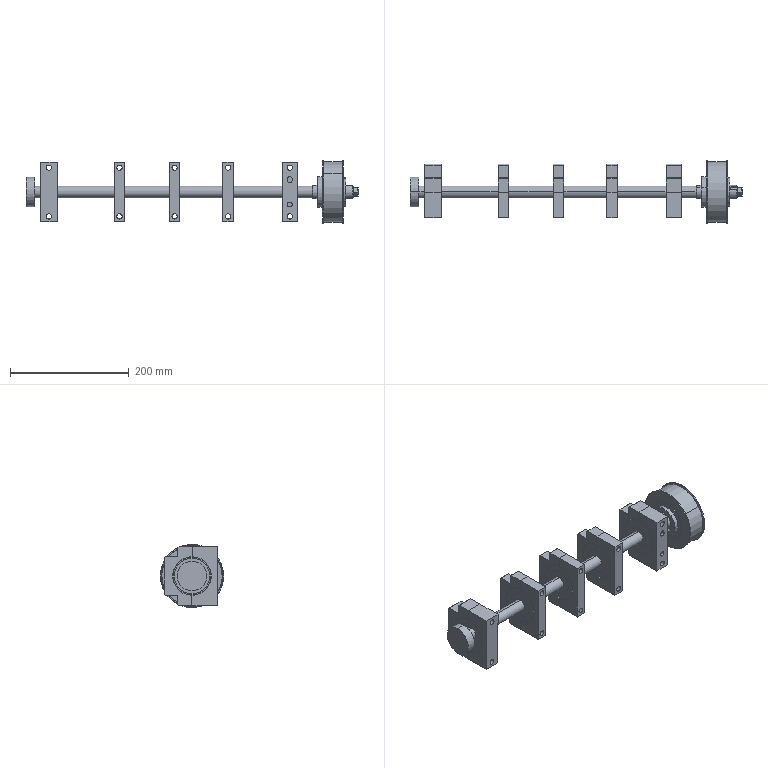Part | SolidWorks | 20 solids | 562 faces | box 559.6 x 107 x 107 mm | volume 1279109 mm3 | cylinder 264 | plane 232 | cone 46 | torus 10 | spline 10 | commonest cylinder face diameters 4 x40 9 x40 60 x20 65 x20 64 x18 20 x14